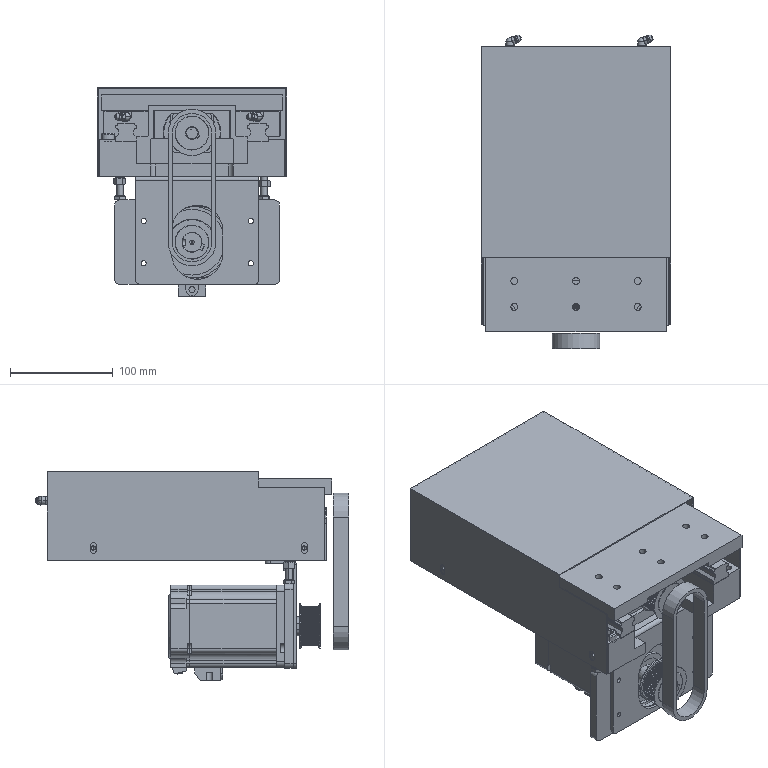Part | SolidWorks | features InContextFeatHolder 15, CompositeCurve 2, Belt 1 | 64 solids | 5474 faces | volume 3170015 mm3 | plane 2695 | cylinder 2309 | cone 398 | spline 24 | sphere 24 | torus 24 | commonest cylinder face diameters 1 x296 0.3 x218 0.56 x206 3.95 x180 0.2 x136 2 x108